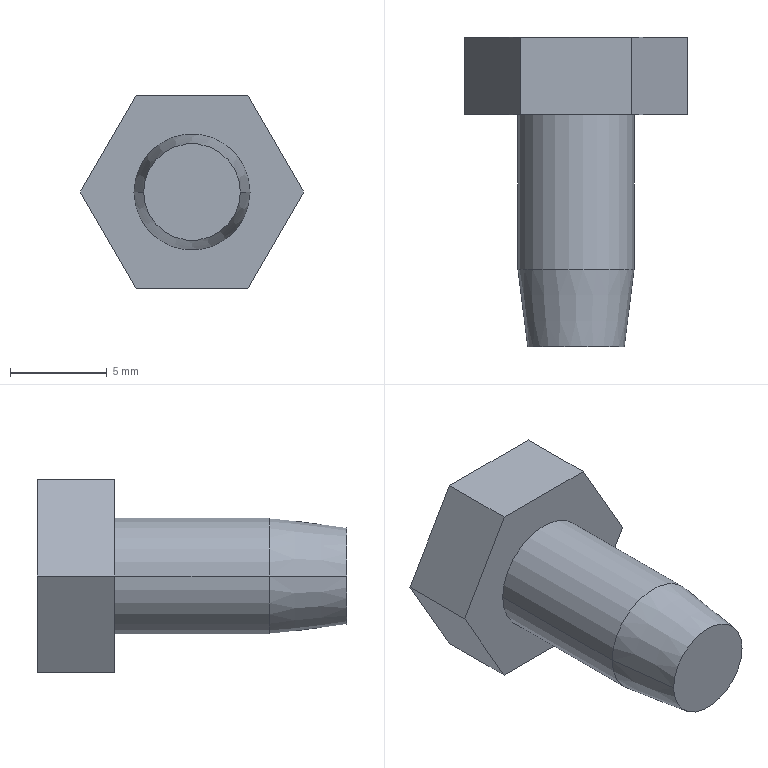Part | STEP file | TAP_SCREW_DIN7500D_M6X12_TORX | 1 solid | 26 faces | box 11.547 x 16 x 10 mm | volume 601.829 mm3 | cylinder 14 | plane 10 | cone 2 | commonest cylinder face diameters 1.007 x6 2 x6 6 x2